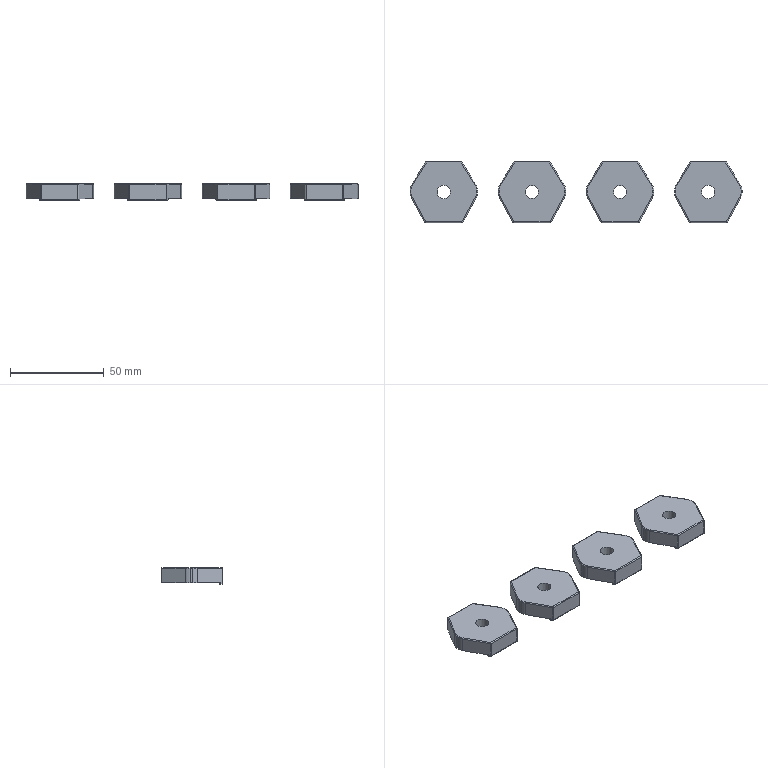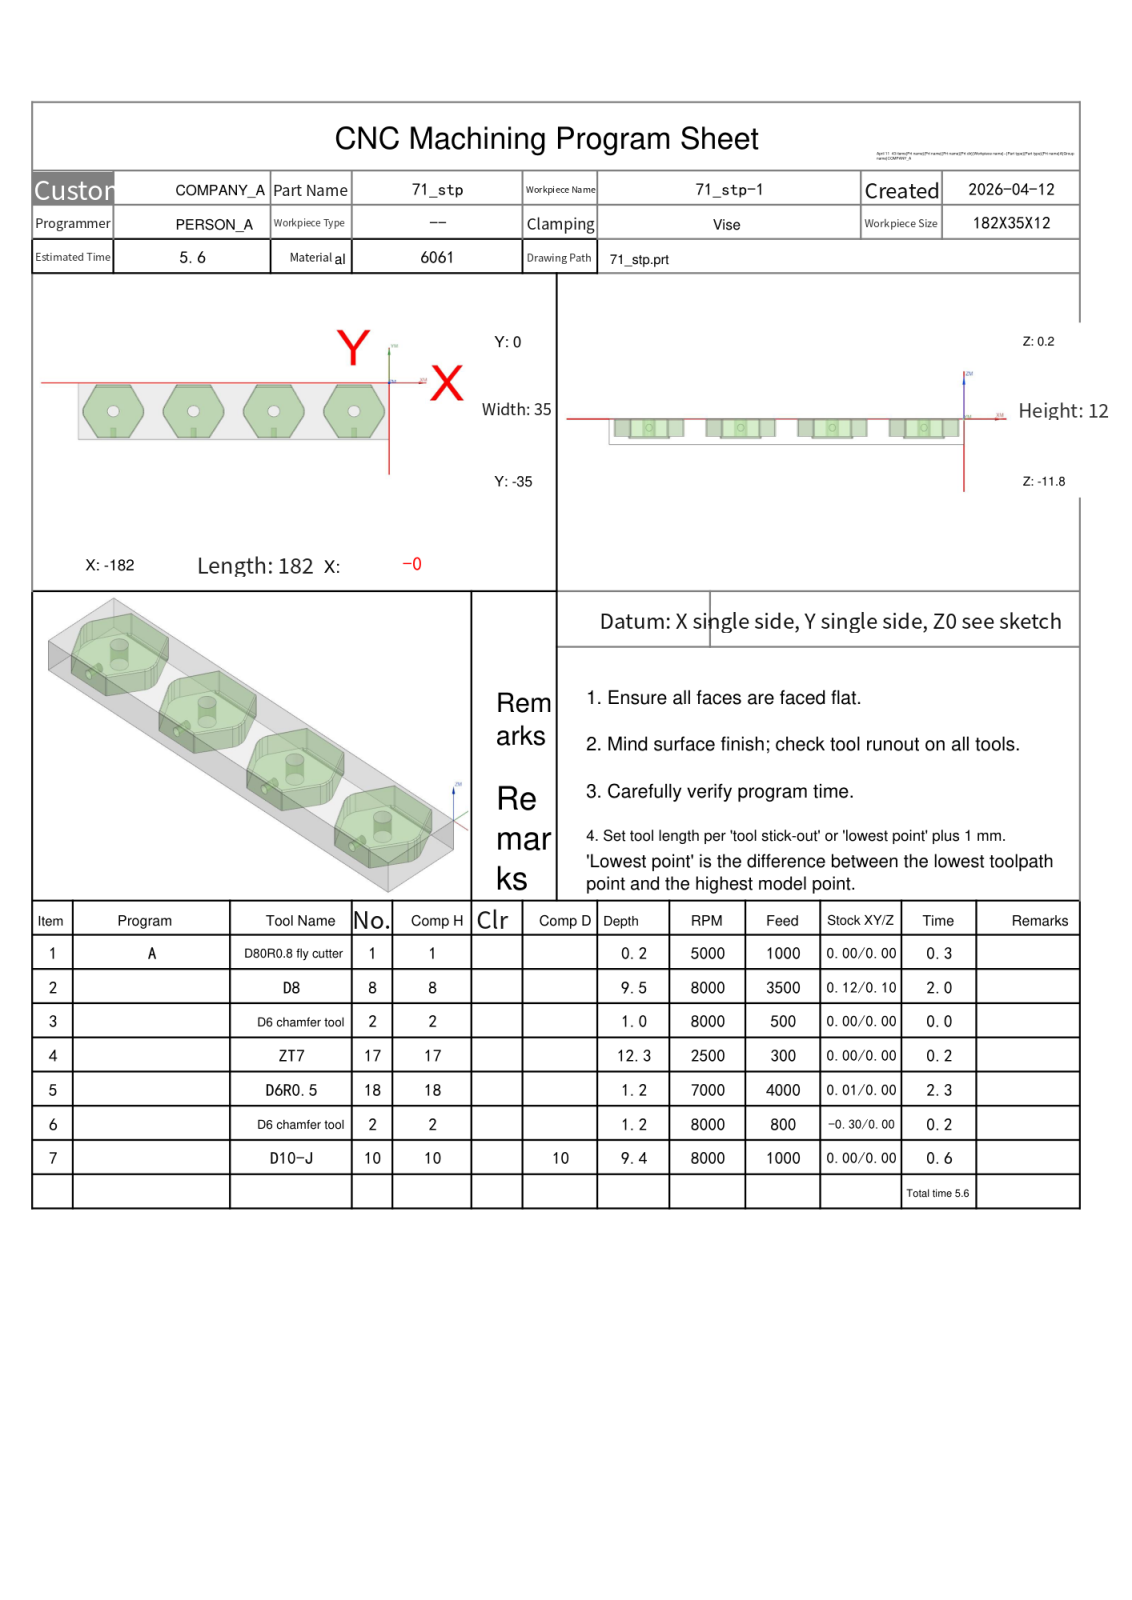NC program | NX | posted by the shop | part box 177 x 33 x 9 mm
Lines 1 to 33 of 15773:
%
O0001
(Machine time: 6.99 MIN)
(===Total Tool:6===)
(T1=D80R0.8 fly cutter D=80.  R=0.8  D-  H01 Z=0.    )
(T8=D8      D=8.   R=0.   D-  H08 Z=-9.3  )
(T2=D6 chamfer tool   D=6.   R=0.   D-  H02 Z=-1.   )
(T17=ZT7    D=7.   DR_a=118 D-  H17 Z=-12.1 )
(T18=D6R0.5 D=6.   R=0.5  D-  H18 Z=-1.   )
(T10=D10-J  D=10.  R=0.   D10 H10 Z=-9.2  )
G80 G90 G17 G49 G40
G91 G28 Z0
M01
N1 T01 M06
(D80R0.8 fly cutter  D=80. R=0.8 H=01 ce=0.00 di=0.00)
(MAX_Z=20. MIN_Z=0. Time=0.28M)
G00 G90 G54 X42.5 Y-17.5 M03 S5000
G43 H01 Z20.
M08
Z2.
G01 Z0.0 F1000.
X37.5
X-219.5
X-224.5
Z2.
G00 Z20.
G91 G28 Z0.0
M05
M09
G91 G28 Z0.0
M01